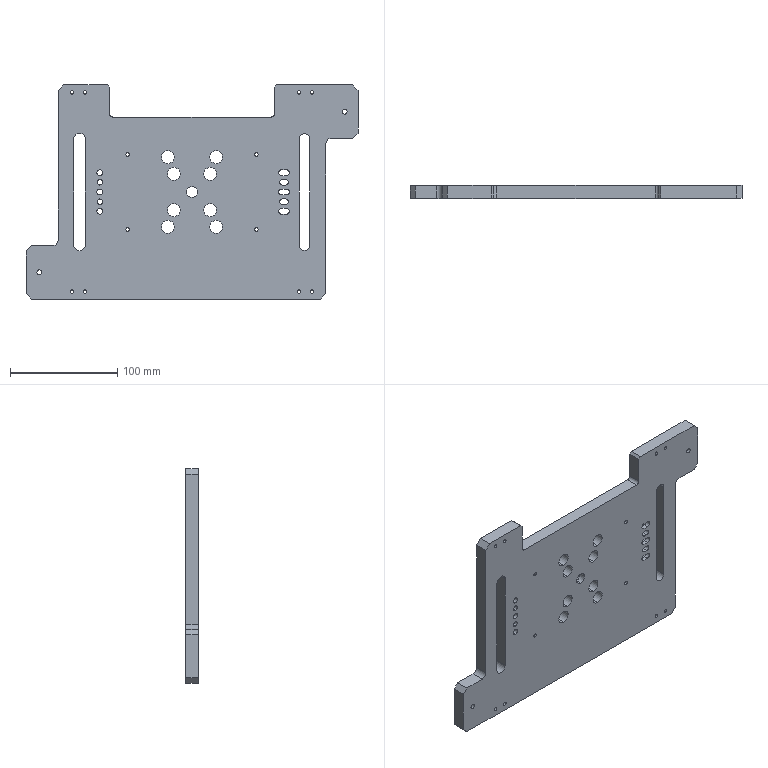Part | STEP file | 1 solid | 149 faces | box 310 x 12 x 200 mm | volume 529543 mm3 | cylinder 94 | plane 51 | cone 4 | commonest cylinder face diameters 3.3 x24 12 x20 10 x17 5.5 x12 5 x8 4.5 x4